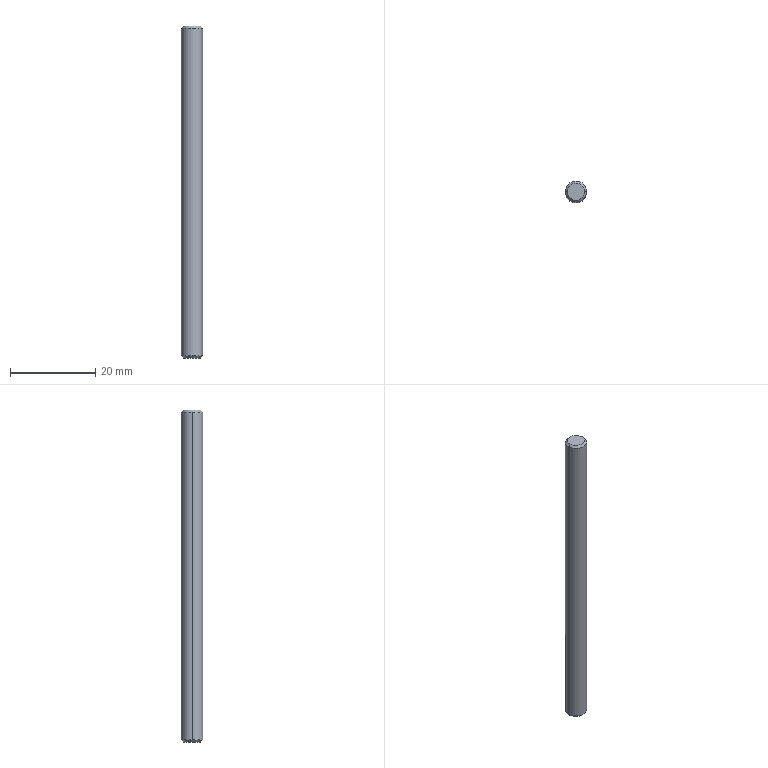Part | SolidWorks | features BaseBody 1 | 1 solid | 8 faces | box 5 x 5 x 78 mm | volume 1528 mm3 | cone 4 | cylinder 2 | plane 2 | commonest cylinder face diameters 5 x2
STEP:
#1=CARTESIAN_POINT('',(2.,4.6,39.));
#2=VERTEX_POINT('',#1);
#3=CARTESIAN_POINT('',(-2.,4.6,39.));
#4=VERTEX_POINT('',#3);
#5=CARTESIAN_POINT('',(0.,4.6,39.));
#6=DIRECTION('',(0.,0.,1.));
#7=DIRECTION('',(1.,0.,0.));
#8=AXIS2_PLACEMENT_3D('',#5,#6,#7);
#9=CIRCLE('',#8,2.);
#10=EDGE_CURVE('',#2,#4,#9,.T.);
#11=ORIENTED_EDGE('',*,*,#10,.F.);
#12=CARTESIAN_POINT('',(2.5,4.6,38.5));
#13=VERTEX_POINT('',#12);
#14=CARTESIAN_POINT('',(2.,4.6,39.));
#15=DIRECTION('',(0.7071,0.,-0.7071));
#16=VECTOR('',#15,1000.);
#17=LINE('',#14,#16);
#18=EDGE_CURVE('',#2,#13,#17,.T.);
#19=ORIENTED_EDGE('',*,*,#18,.T.);
#20=CARTESIAN_POINT('',(-2.5,4.6,38.5));
#21=VERTEX_POINT('',#20);
#22=CARTESIAN_POINT('',(0.,4.6,38.5));
#23=DIRECTION('',(0.,0.,-1.));
#24=DIRECTION('',(1.,0.,0.));
#25=AXIS2_PLACEMENT_3D('',#22,#23,#24);
#26=CIRCLE('',#25,2.5);
#27=EDGE_CURVE('',#21,#13,#26,.T.);
#28=ORIENTED_EDGE('',*,*,#27,.F.);
#29=CARTESIAN_POINT('',(-2.,4.6,39.));
#30=DIRECTION('',(-0.7071,0.,-0.7071));
#31=VECTOR('',#30,1000.);
#32=LINE('',#29,#31);
#33=EDGE_CURVE('',#4,#21,#32,.T.);
#34=ORIENTED_EDGE('',*,*,#33,.F.);
#35=EDGE_LOOP('',(#11,#19,#28,#34));
#36=FACE_OUTER_BOUND('',#35,.T.);
#37=CARTESIAN_POINT('',(0.,4.6,39.));
#38=DIRECTION('',(0.,0.,-1.));
#39=DIRECTION('',(-1.,0.,0.));
#40=AXIS2_PLACEMENT_3D('',#37,#38,#39);
#41=CONICAL_SURFACE('',#40,2.,0.7854);
#42=ADVANCED_FACE('',(#36),#41,.T.);
#43=CARTESIAN_POINT('',(-2.,4.6,-39.));
#44=VERTEX_POINT('',#43);
#45=CARTESIAN_POINT('',(2.,4.6,-39.));
#46=VERTEX_POINT('',#45);
#47=CARTESIAN_POINT('',(0.,4.6,-39.));
#48=DIRECTION('',(0.,0.,-1.));
#49=DIRECTION('',(1.,0.,0.));
#50=AXIS2_PLACEMENT_3D('',#47,#48,#49);
#51=CIRCLE('',#50,2.);
#52=EDGE_CURVE('',#44,#46,#51,.T.);
#53=ORIENTED_EDGE('',*,*,#52,.F.);
#54=CARTESIAN_POINT('',(-2.5,4.6,-38.5));
#55=VERTEX_POINT('',#54);
#56=CARTESIAN_POINT('',(-2.5,4.6,-38.5));
#57=DIRECTION('',(-0.7071,0.,0.7071));
#58=VECTOR('',#57,1000.);
#59=LINE('',#56,#58);
#60=EDGE_CURVE('',#44,#55,#59,.T.);
#61=ORIENTED_EDGE('',*,*,#60,.T.);
#62=CARTESIAN_POINT('',(2.5,4.6,-38.5));
#63=VERTEX_POINT('',#62);
#64=CARTESIAN_POINT('',(0.,4.6,-38.5));
#65=DIRECTION('',(0.,0.,1.));
#66=DIRECTION('',(1.,0.,0.));
#67=AXIS2_PLACEMENT_3D('',#64,#65,#66);
#68=CIRCLE('',#67,2.5);
#69=EDGE_CURVE('',#63,#55,#68,.T.);
#70=ORIENTED_EDGE('',*,*,#69,.F.);
#71=CARTESIAN_POINT('',(2.5,4.6,-38.5));
#72=DIRECTION('',(0.7071,0.,0.7071));
#73=VECTOR('',#72,1000.);
#74=LINE('',#71,#73);
#75=EDGE_CURVE('',#46,#63,#74,.T.);
#76=ORIENTED_EDGE('',*,*,#75,.F.);
#77=EDGE_LOOP('',(#53,#61,#70,#76));
#78=FACE_OUTER_BOUND('',#77,.T.);
#79=CARTESIAN_POINT('',(0.,4.6,-38.5));
#80=DIRECTION('',(0.,0.,1.));
#81=DIRECTION('',(1.,0.,0.));
#82=AXIS2_PLACEMENT_3D('',#79,#80,#81);
#83=CONICAL_SURFACE('',#82,2.5,0.7854);
#84=ADVANCED_FACE('',(#78),#83,.T.);
#85=ORIENTED_EDGE('',*,*,#27,.T.);
#86=CARTESIAN_POINT('',(2.5,4.6,39.));
#87=DIRECTION('',(0.,0.,-1.));
#88=VECTOR('',#87,1000.);
#89=LINE('',#86,#88);
#90=EDGE_CURVE('',#13,#63,#89,.T.);
#91=ORIENTED_EDGE('',*,*,#90,.T.);
#92=ORIENTED_EDGE('',*,*,#69,.T.);
#93=CARTESIAN_POINT('',(-2.5,4.6,39.));
#94=DIRECTION('',(0.,0.,-1.));
#95=VECTOR('',#94,1000.);
#96=LINE('',#93,#95);
#97=EDGE_CURVE('',#21,#55,#96,.T.);
#98=ORIENTED_EDGE('',*,*,#97,.F.);
#99=EDGE_LOOP('',(#85,#91,#92,#98));
#100=FACE_OUTER_BOUND('',#99,.T.);
#101=CARTESIAN_POINT('',(0.,4.6,39.));
#102=DIRECTION('',(0.,0.,-1.));
#103=DIRECTION('',(-1.,0.,0.));
#104=AXIS2_PLACEMENT_3D('',#101,#102,#103);
#105=CYLINDRICAL_SURFACE('',#104,2.5);
#106=ADVANCED_FACE('',(#100),#105,.T.);
#107=ORIENTED_EDGE('',*,*,#90,.F.);
#108=CARTESIAN_POINT('',(0.,4.6,38.5));
#109=DIRECTION('',(0.,0.,-1.));
#110=DIRECTION('',(1.,0.,0.));
#111=AXIS2_PLACEMENT_3D('',#108,#109,#110);
#112=CIRCLE('',#111,2.5);
#113=EDGE_CURVE('',#13,#21,#112,.T.);
#114=ORIENTED_EDGE('',*,*,#113,.T.);
#115=ORIENTED_EDGE('',*,*,#97,.T.);
#116=CARTESIAN_POINT('',(0.,4.6,-38.5));
#117=DIRECTION('',(0.,0.,1.));
#118=DIRECTION('',(1.,0.,0.));
#119=AXIS2_PLACEMENT_3D('',#116,#117,#118);
#120=CIRCLE('',#119,2.5);
#121=EDGE_CURVE('',#55,#63,#120,.T.);
#122=ORIENTED_EDGE('',*,*,#121,.T.);
#123=EDGE_LOOP('',(#107,#114,#115,#122));
#124=FACE_OUTER_BOUND('',#123,.T.);
#125=CARTESIAN_POINT('',(0.,4.6,39.));
#126=DIRECTION('',(0.,0.,-1.));
#127=DIRECTION('',(-1.,0.,0.));
#128=AXIS2_PLACEMENT_3D('',#125,#126,#127);
#129=CYLINDRICAL_SURFACE('',#128,2.5);
#130=ADVANCED_FACE('',(#124),#129,.T.);
#131=CARTESIAN_POINT('',(0.,4.6,39.));
#132=DIRECTION('',(0.,0.,1.));
#133=DIRECTION('',(1.,0.,0.));
#134=AXIS2_PLACEMENT_3D('',#131,#132,#133);
#135=CIRCLE('',#134,2.);
#136=EDGE_CURVE('',#4,#2,#135,.T.);
#137=ORIENTED_EDGE('',*,*,#136,.T.);
#138=ORIENTED_EDGE('',*,*,#10,.T.);
#139=EDGE_LOOP('',(#137,#138));
#140=FACE_OUTER_BOUND('',#139,.T.);
#141=CARTESIAN_POINT('',(0.,4.6,39.));
#142=DIRECTION('',(0.,0.,1.));
#143=DIRECTION('',(1.,0.,0.));
#144=AXIS2_PLACEMENT_3D('',#141,#142,#143);
#145=PLANE('',#144);
#146=ADVANCED_FACE('',(#140),#145,.T.);
#147=CARTESIAN_POINT('',(0.,4.6,-39.));
#148=DIRECTION('',(0.,0.,-1.));
#149=DIRECTION('',(1.,0.,0.));
#150=AXIS2_PLACEMENT_3D('',#147,#148,#149);
#151=CIRCLE('',#150,2.);
#152=EDGE_CURVE('',#46,#44,#151,.T.);
#153=ORIENTED_EDGE('',*,*,#152,.T.);
#154=ORIENTED_EDGE('',*,*,#52,.T.);
#155=EDGE_LOOP('',(#153,#154));
#156=FACE_OUTER_BOUND('',#155,.T.);
#157=CARTESIAN_POINT('',(0.,4.6,-39.));
#158=DIRECTION('',(0.,0.,1.));
#159=DIRECTION('',(1.,0.,0.));
#160=AXIS2_PLACEMENT_3D('',#157,#158,#159);
#161=PLANE('',#160);
#162=ADVANCED_FACE('',(#156),#161,.F.);
#163=ORIENTED_EDGE('',*,*,#60,.F.);
#164=ORIENTED_EDGE('',*,*,#152,.F.);
#165=ORIENTED_EDGE('',*,*,#75,.T.);
#166=ORIENTED_EDGE('',*,*,#121,.F.);
#167=EDGE_LOOP('',(#163,#164,#165,#166));
#168=FACE_OUTER_BOUND('',#167,.T.);
#169=CARTESIAN_POINT('',(0.,4.6,-38.5));
#170=DIRECTION('',(0.,0.,1.));
#171=DIRECTION('',(1.,0.,0.));
#172=AXIS2_PLACEMENT_3D('',#169,#170,#171);
#173=CONICAL_SURFACE('',#172,2.5,0.7854);
#174=ADVANCED_FACE('',(#168),#173,.T.);
#175=ORIENTED_EDGE('',*,*,#18,.F.);
#176=ORIENTED_EDGE('',*,*,#136,.F.);
#177=ORIENTED_EDGE('',*,*,#33,.T.);
#178=ORIENTED_EDGE('',*,*,#113,.F.);
#179=EDGE_LOOP('',(#175,#176,#177,#178));
#180=FACE_OUTER_BOUND('',#179,.T.);
#181=CARTESIAN_POINT('',(0.,4.6,39.));
#182=DIRECTION('',(0.,0.,-1.));
#183=DIRECTION('',(-1.,0.,0.));
#184=AXIS2_PLACEMENT_3D('',#181,#182,#183);
#185=CONICAL_SURFACE('',#184,2.,0.7854);
#186=ADVANCED_FACE('',(#180),#185,.T.);
#187=CLOSED_SHELL('',(#42,#84,#106,#130,#146,#162,#174,#186));
#188=MANIFOLD_SOLID_BREP('',#187);
#189=CARTESIAN_POINT('',(0.,0.,0.));
#190=DIRECTION('',(0.,0.,1.));
#191=DIRECTION('',(1.,0.,0.));
#192=AXIS2_PLACEMENT_3D('',#189,#190,#191);
#193=(LENGTH_UNIT()NAMED_UNIT(*)SI_UNIT(.MILLI.,.METRE.));
#194=UNCERTAINTY_MEASURE_WITH_UNIT(LENGTH_MEASURE(0.00001),#193,'','');
#195=(NAMED_UNIT(*)PLANE_ANGLE_UNIT()SI_UNIT($,.RADIAN.));
#196=(NAMED_UNIT(*)SI_UNIT($,.STERADIAN.)SOLID_ANGLE_UNIT());
#197=(GEOMETRIC_REPRESENTATION_CONTEXT(3)GLOBAL_UNCERTAINTY_ASSIGNED_CONTEXT((#194))GLOBAL_UNIT_ASSIGNED_CONTEXT((#193,#195,#196))REPRESENTATION_CONTEXT('',''));
#198=ADVANCED_BREP_SHAPE_REPRESENTATION('',(#188,#192),#197);